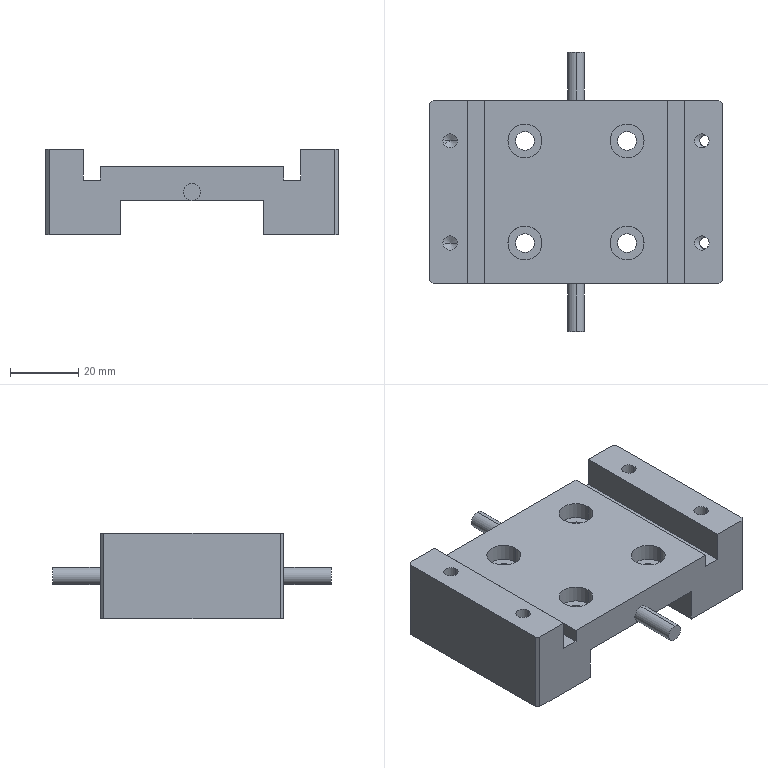Part | NX | features BREP 1 | 1 solid | 68 faces | box 86 x 82 x 25 mm | volume 71512 mm3 | cylinder 32 | plane 28 | cone 8 | commonest cylinder face diameters 4.2 x8 5.5 x8 10 x8 3.3 x4 5 x4